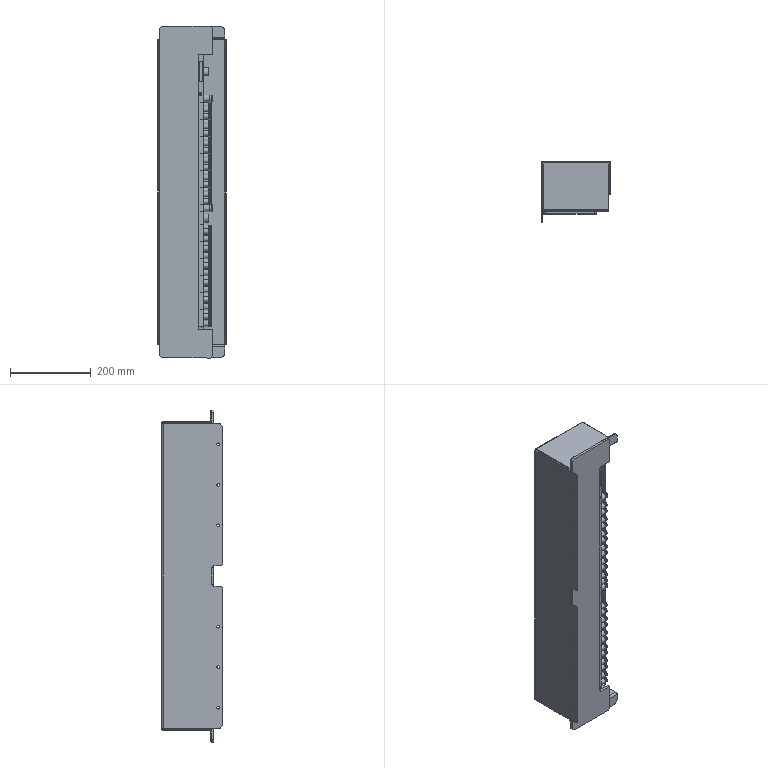Part | NX | features BREP 150 | 150 solids | 11465 faces | volume 4723286 mm3 | plane 7094 | cylinder 2922 | cone 854 | torus 553 | sphere 42 | commonest cylinder face diameters 5.3 x336 1 x239 2 x178 3.6 x126 8 x116 11.4 x98